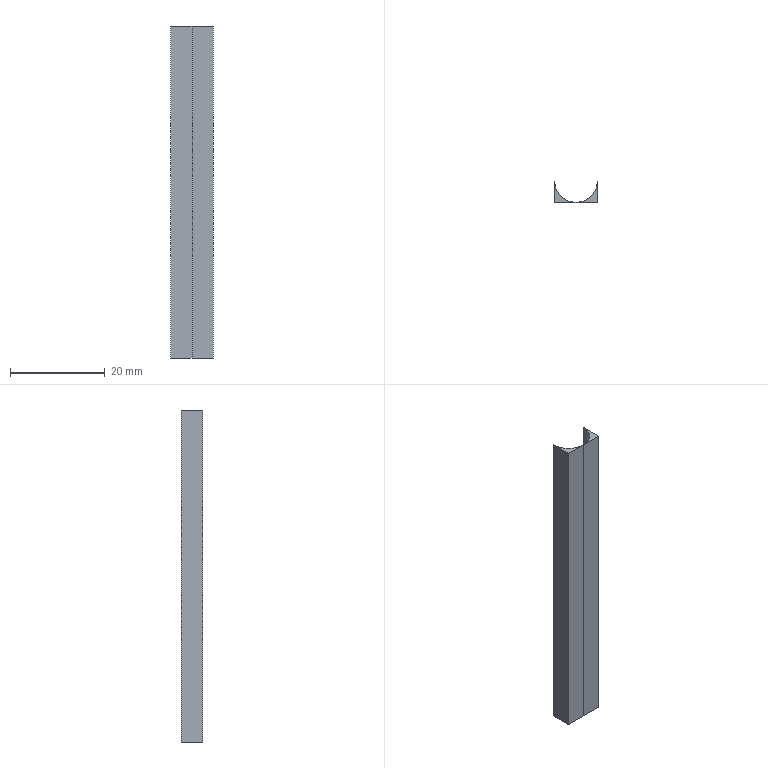Part | STEP file | DCV-000-W03_1 | 2 solids | 10 faces | box 9 x 4.5 x 70 mm | volume 608.396 mm3 | plane 8 | cylinder 2 | commonest cylinder face diameters 9 x2
STEP:
#1=CARTESIAN_POINT('',(0.,0.,0.));
#2=DIRECTION('',(0.,0.,1.));
#3=DIRECTION('',(1.,0.,0.));
#4=AXIS2_PLACEMENT_3D('',#1,#2,#3);
#5=CARTESIAN_POINT('',(0.,-4.5,236.));
#6=VERTEX_POINT('',#5);
#7=CARTESIAN_POINT('',(4.5,0.,236.));
#8=VERTEX_POINT('',#7);
#9=CARTESIAN_POINT('',(0.,0.,236.));
#10=DIRECTION('',(0.,0.,1.));
#11=DIRECTION('',(1.,0.,0.));
#12=AXIS2_PLACEMENT_3D('',#9,#10,#11);
#13=CIRCLE('',#12,4.5);
#14=CARTESIAN_POINT('',(20.,-4.5,236.));
#15=DIRECTION('',(0.,0.,1.));
#16=DIRECTION('',(1.,0.,0.));
#17=AXIS2_PLACEMENT_3D('',#14,#15,#16);
#18=PLANE('',#17);
#19=CARTESIAN_POINT('',(-20.,4.5));
#20=DIRECTION('',(1.,0.));
#21=AXIS2_PLACEMENT_2D('',#19,#20);
#22=CIRCLE('',#21,4.5);
#23=(GEOMETRIC_REPRESENTATION_CONTEXT(2)PARAMETRIC_REPRESENTATION_CONTEXT()REPRESENTATION_CONTEXT('',''));
#24=DEFINITIONAL_REPRESENTATION('',(#22),#23);
#25=PCURVE('',#18,#24);
#26=CARTESIAN_POINT('',(0.,0.,0.));
#27=DIRECTION('',(0.,0.,1.));
#28=DIRECTION('',(1.,0.,0.));
#29=AXIS2_PLACEMENT_3D('',#26,#27,#28);
#30=CYLINDRICAL_SURFACE('',#29,4.5);
#31=CARTESIAN_POINT('',(0.,236.));
#32=DIRECTION('',(1.,0.));
#33=VECTOR('',#32,1.);
#34=LINE('',#31,#33);
#35=(GEOMETRIC_REPRESENTATION_CONTEXT(2)PARAMETRIC_REPRESENTATION_CONTEXT()REPRESENTATION_CONTEXT('',''));
#36=DEFINITIONAL_REPRESENTATION('',(#34),#35);
#37=PCURVE('',#30,#36);
#38=SURFACE_CURVE('',#13,(#25,#37),.PCURVE_S1.);
#39=EDGE_CURVE('',#6,#8,#38,.T.);
#40=ORIENTED_EDGE('',*,*,#39,.F.);
#41=CARTESIAN_POINT('',(4.5,-4.5,236.));
#42=VERTEX_POINT('',#41);
#43=CARTESIAN_POINT('',(25.,-4.5,236.));
#44=DIRECTION('',(-1.,0.,0.));
#45=VECTOR('',#44,1.);
#46=LINE('',#43,#45);
#47=CARTESIAN_POINT('',(5.,0.));
#48=DIRECTION('',(-1.,0.));
#49=VECTOR('',#48,1.);
#50=LINE('',#47,#49);
#51=(GEOMETRIC_REPRESENTATION_CONTEXT(2)PARAMETRIC_REPRESENTATION_CONTEXT()REPRESENTATION_CONTEXT('',''));
#52=DEFINITIONAL_REPRESENTATION('',(#50),#51);
#53=PCURVE('',#18,#52);
#54=CARTESIAN_POINT('',(0.,-4.5,201.));
#55=DIRECTION('',(0.,-1.,0.));
#56=DIRECTION('',(0.,0.,-1.));
#57=AXIS2_PLACEMENT_3D('',#54,#55,#56);
#58=PLANE('',#57);
#59=CARTESIAN_POINT('',(-35.,25.));
#60=DIRECTION('',(0.,-1.));
#61=VECTOR('',#60,1.);
#62=LINE('',#59,#61);
#63=(GEOMETRIC_REPRESENTATION_CONTEXT(2)PARAMETRIC_REPRESENTATION_CONTEXT()REPRESENTATION_CONTEXT('',''));
#64=DEFINITIONAL_REPRESENTATION('',(#62),#63);
#65=PCURVE('',#58,#64);
#66=SURFACE_CURVE('',#46,(#53,#65),.PCURVE_S1.);
#67=EDGE_CURVE('',#42,#6,#66,.T.);
#68=ORIENTED_EDGE('',*,*,#67,.F.);
#69=CARTESIAN_POINT('',(4.5,-2.25,236.));
#70=DIRECTION('',(0.,-1.,0.));
#71=VECTOR('',#70,1.);
#72=LINE('',#69,#71);
#73=CARTESIAN_POINT('',(-15.5,2.25));
#74=DIRECTION('',(0.,-1.));
#75=VECTOR('',#74,1.);
#76=LINE('',#73,#75);
#77=(GEOMETRIC_REPRESENTATION_CONTEXT(2)PARAMETRIC_REPRESENTATION_CONTEXT()REPRESENTATION_CONTEXT('',''));
#78=DEFINITIONAL_REPRESENTATION('',(#76),#77);
#79=PCURVE('',#18,#78);
#80=CARTESIAN_POINT('',(4.5,0.,0.));
#81=DIRECTION('',(1.,0.,0.));
#82=DIRECTION('',(0.,1.,0.));
#83=AXIS2_PLACEMENT_3D('',#80,#81,#82);
#84=PLANE('',#83);
#85=CARTESIAN_POINT('',(-2.25,236.));
#86=DIRECTION('',(-1.,0.));
#87=VECTOR('',#86,1.);
#88=LINE('',#85,#87);
#89=(GEOMETRIC_REPRESENTATION_CONTEXT(2)PARAMETRIC_REPRESENTATION_CONTEXT()REPRESENTATION_CONTEXT('',''));
#90=DEFINITIONAL_REPRESENTATION('',(#88),#89);
#91=PCURVE('',#84,#90);
#92=SURFACE_CURVE('',#72,(#79,#91),.PCURVE_S1.);
#93=EDGE_CURVE('',#8,#42,#92,.T.);
#94=ORIENTED_EDGE('',*,*,#93,.F.);
#95=EDGE_LOOP('',(#40,#68,#94));
#96=FACE_BOUND('',#95,.T.);
#97=ADVANCED_FACE('',(#96),#18,.T.);
#98=CARTESIAN_POINT('',(4.5,-4.5,166.));
#99=VERTEX_POINT('',#98);
#100=CARTESIAN_POINT('',(4.5,-4.5,100.5));
#101=DIRECTION('',(0.,0.,-1.));
#102=VECTOR('',#101,1.);
#103=LINE('',#100,#102);
#104=CARTESIAN_POINT('',(100.5,4.5));
#105=DIRECTION('',(1.,0.));
#106=VECTOR('',#105,1.);
#107=LINE('',#104,#106);
#108=(GEOMETRIC_REPRESENTATION_CONTEXT(2)PARAMETRIC_REPRESENTATION_CONTEXT()REPRESENTATION_CONTEXT('',''));
#109=DEFINITIONAL_REPRESENTATION('',(#107),#108);
#110=PCURVE('',#58,#109);
#111=CARTESIAN_POINT('',(-4.5,100.5));
#112=DIRECTION('',(0.,-1.));
#113=VECTOR('',#112,1.);
#114=LINE('',#111,#113);
#115=(GEOMETRIC_REPRESENTATION_CONTEXT(2)PARAMETRIC_REPRESENTATION_CONTEXT()REPRESENTATION_CONTEXT('',''));
#116=DEFINITIONAL_REPRESENTATION('',(#114),#115);
#117=PCURVE('',#84,#116);
#118=SURFACE_CURVE('',#103,(#110,#117),.PCURVE_S1.);
#119=EDGE_CURVE('',#42,#99,#118,.T.);
#120=ORIENTED_EDGE('',*,*,#119,.F.);
#121=ORIENTED_EDGE('',*,*,#67,.T.);
#122=CARTESIAN_POINT('',(0.,-4.5,166.));
#123=VERTEX_POINT('',#122);
#124=CARTESIAN_POINT('',(0.,-4.5,0.));
#125=DIRECTION('',(0.,0.,1.));
#126=VECTOR('',#125,1.);
#127=LINE('',#124,#126);
#128=CARTESIAN_POINT('',(201.,0.));
#129=DIRECTION('',(-1.,0.));
#130=VECTOR('',#129,1.);
#131=LINE('',#128,#130);
#132=(GEOMETRIC_REPRESENTATION_CONTEXT(2)PARAMETRIC_REPRESENTATION_CONTEXT()REPRESENTATION_CONTEXT('',''));
#133=DEFINITIONAL_REPRESENTATION('',(#131),#132);
#134=PCURVE('',#58,#133);
#135=CARTESIAN_POINT('',(4.712,0.));
#136=DIRECTION('',(0.,1.));
#137=VECTOR('',#136,1.);
#138=LINE('',#135,#137);
#139=(GEOMETRIC_REPRESENTATION_CONTEXT(2)PARAMETRIC_REPRESENTATION_CONTEXT()REPRESENTATION_CONTEXT('',''));
#140=DEFINITIONAL_REPRESENTATION('',(#138),#139);
#141=PCURVE('',#30,#140);
#142=SURFACE_CURVE('',#127,(#134,#141),.PCURVE_S1.);
#143=EDGE_CURVE('',#123,#6,#142,.T.);
#144=ORIENTED_EDGE('',*,*,#143,.F.);
#145=CARTESIAN_POINT('',(-25.,-4.5,166.));
#146=DIRECTION('',(1.,0.,0.));
#147=VECTOR('',#146,1.);
#148=LINE('',#145,#147);
#149=CARTESIAN_POINT('',(35.,-25.));
#150=DIRECTION('',(0.,1.));
#151=VECTOR('',#150,1.);
#152=LINE('',#149,#151);
#153=(GEOMETRIC_REPRESENTATION_CONTEXT(2)PARAMETRIC_REPRESENTATION_CONTEXT()REPRESENTATION_CONTEXT('',''));
#154=DEFINITIONAL_REPRESENTATION('',(#152),#153);
#155=PCURVE('',#58,#154);
#156=CARTESIAN_POINT('',(0.,-4.5,166.));
#157=DIRECTION('',(0.,0.,-1.));
#158=DIRECTION('',(0.,-1.,0.));
#159=AXIS2_PLACEMENT_3D('',#156,#157,#158);
#160=PLANE('',#159);
#161=CARTESIAN_POINT('',(0.,25.));
#162=DIRECTION('',(0.,-1.));
#163=VECTOR('',#162,1.);
#164=LINE('',#161,#163);
#165=(GEOMETRIC_REPRESENTATION_CONTEXT(2)PARAMETRIC_REPRESENTATION_CONTEXT()REPRESENTATION_CONTEXT('',''));
#166=DEFINITIONAL_REPRESENTATION('',(#164),#165);
#167=PCURVE('',#160,#166);
#168=SURFACE_CURVE('',#148,(#155,#167),.PCURVE_S1.);
#169=EDGE_CURVE('',#123,#99,#168,.T.);
#170=ORIENTED_EDGE('',*,*,#169,.T.);
#171=EDGE_LOOP('',(#120,#121,#144,#170));
#172=FACE_BOUND('',#171,.T.);
#173=ADVANCED_FACE('',(#172),#58,.T.);
#174=CARTESIAN_POINT('',(4.5,0.,166.));
#175=VERTEX_POINT('',#174);
#176=CARTESIAN_POINT('',(0.,0.,166.));
#177=DIRECTION('',(0.,0.,-1.));
#178=DIRECTION('',(1.,0.,0.));
#179=AXIS2_PLACEMENT_3D('',#176,#177,#178);
#180=CIRCLE('',#179,4.5);
#181=CARTESIAN_POINT('',(-4.5,0.));
#182=DIRECTION('',(0.,-1.));
#183=AXIS2_PLACEMENT_2D('',#181,#182);
#184=CIRCLE('',#183,4.5);
#185=(GEOMETRIC_REPRESENTATION_CONTEXT(2)PARAMETRIC_REPRESENTATION_CONTEXT()REPRESENTATION_CONTEXT('',''));
#186=DEFINITIONAL_REPRESENTATION('',(#184),#185);
#187=PCURVE('',#160,#186);
#188=CARTESIAN_POINT('',(6.283,166.));
#189=DIRECTION('',(-1.,0.));
#190=VECTOR('',#189,1.);
#191=LINE('',#188,#190);
#192=(GEOMETRIC_REPRESENTATION_CONTEXT(2)PARAMETRIC_REPRESENTATION_CONTEXT()REPRESENTATION_CONTEXT('',''));
#193=DEFINITIONAL_REPRESENTATION('',(#191),#192);
#194=PCURVE('',#30,#193);
#195=SURFACE_CURVE('',#180,(#187,#194),.PCURVE_S1.);
#196=EDGE_CURVE('',#175,#123,#195,.T.);
#197=ORIENTED_EDGE('',*,*,#196,.F.);
#198=CARTESIAN_POINT('',(4.5,-2.25,166.));
#199=DIRECTION('',(0.,1.,0.));
#200=VECTOR('',#199,1.);
#201=LINE('',#198,#200);
#202=CARTESIAN_POINT('',(-2.25,-4.5));
#203=DIRECTION('',(-1.,0.));
#204=VECTOR('',#203,1.);
#205=LINE('',#202,#204);
#206=(GEOMETRIC_REPRESENTATION_CONTEXT(2)PARAMETRIC_REPRESENTATION_CONTEXT()REPRESENTATION_CONTEXT('',''));
#207=DEFINITIONAL_REPRESENTATION('',(#205),#206);
#208=PCURVE('',#160,#207);
#209=CARTESIAN_POINT('',(-2.25,166.));
#210=DIRECTION('',(1.,0.));
#211=VECTOR('',#210,1.);
#212=LINE('',#209,#211);
#213=(GEOMETRIC_REPRESENTATION_CONTEXT(2)PARAMETRIC_REPRESENTATION_CONTEXT()REPRESENTATION_CONTEXT('',''));
#214=DEFINITIONAL_REPRESENTATION('',(#212),#213);
#215=PCURVE('',#84,#214);
#216=SURFACE_CURVE('',#201,(#208,#215),.PCURVE_S1.);
#217=EDGE_CURVE('',#99,#175,#216,.T.);
#218=ORIENTED_EDGE('',*,*,#217,.F.);
#219=ORIENTED_EDGE('',*,*,#169,.F.);
#220=EDGE_LOOP('',(#197,#218,#219));
#221=FACE_BOUND('',#220,.T.);
#222=ADVANCED_FACE('',(#221),#160,.T.);
#223=ORIENTED_EDGE('',*,*,#217,.T.);
#224=CARTESIAN_POINT('',(4.5,0.,0.));
#225=DIRECTION('',(0.,0.,1.));
#226=VECTOR('',#225,1.);
#227=LINE('',#224,#226);
#228=CARTESIAN_POINT('',(0.,0.));
#229=DIRECTION('',(0.,1.));
#230=VECTOR('',#229,1.);
#231=LINE('',#228,#230);
#232=(GEOMETRIC_REPRESENTATION_CONTEXT(2)PARAMETRIC_REPRESENTATION_CONTEXT()REPRESENTATION_CONTEXT('',''));
#233=DEFINITIONAL_REPRESENTATION('',(#231),#232);
#234=PCURVE('',#84,#233);
#235=CARTESIAN_POINT('',(6.283,0.));
#236=DIRECTION('',(0.,1.));
#237=VECTOR('',#236,1.);
#238=LINE('',#235,#237);
#239=(GEOMETRIC_REPRESENTATION_CONTEXT(2)PARAMETRIC_REPRESENTATION_CONTEXT()REPRESENTATION_CONTEXT('',''));
#240=DEFINITIONAL_REPRESENTATION('',(#238),#239);
#241=PCURVE('',#30,#240);
#242=SURFACE_CURVE('',#227,(#234,#241),.PCURVE_S1.);
#243=EDGE_CURVE('',#175,#8,#242,.T.);
#244=ORIENTED_EDGE('',*,*,#243,.T.);
#245=ORIENTED_EDGE('',*,*,#93,.T.);
#246=ORIENTED_EDGE('',*,*,#119,.T.);
#247=EDGE_LOOP('',(#223,#244,#245,#246));
#248=FACE_BOUND('',#247,.T.);
#249=ADVANCED_FACE('',(#248),#84,.T.);
#250=ORIENTED_EDGE('',*,*,#243,.T.);
#251=ORIENTED_EDGE('',*,*,#39,.F.);
#252=ORIENTED_EDGE('',*,*,#143,.F.);
#253=ORIENTED_EDGE('',*,*,#196,.F.);
#254=EDGE_LOOP('',(#250,#251,#252,#253));
#255=FACE_BOUND('',#254,.F.);
#256=ADVANCED_FACE('',(#255),#30,.F.);
#257=CLOSED_SHELL('',(#97,#173,#222,#249,#256));
#258=MANIFOLD_SOLID_BREP('',#257);
#259=CARTESIAN_POINT('',(-4.5,0.,236.));
#260=VERTEX_POINT('',#259);
#261=CARTESIAN_POINT('',(0.,-4.5,236.));
#262=VERTEX_POINT('',#261);
#263=CARTESIAN_POINT('',(0.,0.,236.));
#264=DIRECTION('',(0.,0.,1.));
#265=DIRECTION('',(1.,0.,0.));
#266=AXIS2_PLACEMENT_3D('',#263,#264,#265);
#267=CIRCLE('',#266,4.5);
#268=CARTESIAN_POINT('',(0.,0.,0.));
#269=DIRECTION('',(0.,0.,1.));
#270=DIRECTION('',(1.,0.,0.));
#271=AXIS2_PLACEMENT_3D('',#268,#269,#270);
#272=CYLINDRICAL_SURFACE('',#271,4.5);
#273=CARTESIAN_POINT('',(0.,236.));
#274=DIRECTION('',(1.,0.));
#275=VECTOR('',#274,1.);
#276=LINE('',#273,#275);
#277=(GEOMETRIC_REPRESENTATION_CONTEXT(2)PARAMETRIC_REPRESENTATION_CONTEXT()REPRESENTATION_CONTEXT('',''));
#278=DEFINITIONAL_REPRESENTATION('',(#276),#277);
#279=PCURVE('',#272,#278);
#280=CARTESIAN_POINT('',(0.,-4.5,236.));
#281=DIRECTION('',(0.,0.,1.));
#282=DIRECTION('',(1.,0.,0.));
#283=AXIS2_PLACEMENT_3D('',#280,#281,#282);
#284=PLANE('',#283);
#285=CARTESIAN_POINT('',(0.,4.5));
#286=DIRECTION('',(1.,0.));
#287=AXIS2_PLACEMENT_2D('',#285,#286);
#288=CIRCLE('',#287,4.5);
#289=(GEOMETRIC_REPRESENTATION_CONTEXT(2)PARAMETRIC_REPRESENTATION_CONTEXT()REPRESENTATION_CONTEXT('',''));
#290=DEFINITIONAL_REPRESENTATION('',(#288),#289);
#291=PCURVE('',#284,#290);
#292=SURFACE_CURVE('',#267,(#279,#291),.PCURVE_S1.);
#293=EDGE_CURVE('',#260,#262,#292,.T.);
#294=ORIENTED_EDGE('',*,*,#293,.F.);
#295=CARTESIAN_POINT('',(-4.5,0.,166.));
#296=VERTEX_POINT('',#295);
#297=CARTESIAN_POINT('',(-4.5,0.,0.));
#298=DIRECTION('',(0.,0.,-1.));
#299=VECTOR('',#298,1.);
#300=LINE('',#297,#299);
#301=CARTESIAN_POINT('',(3.142,0.));
#302=DIRECTION('',(0.,-1.));
#303=VECTOR('',#302,1.);
#304=LINE('',#301,#303);
#305=(GEOMETRIC_REPRESENTATION_CONTEXT(2)PARAMETRIC_REPRESENTATION_CONTEXT()REPRESENTATION_CONTEXT('',''));
#306=DEFINITIONAL_REPRESENTATION('',(#304),#305);
#307=PCURVE('',#272,#306);
#308=CARTESIAN_POINT('',(-4.5,0.,236.));
#309=DIRECTION('',(-1.,0.,0.));
#310=DIRECTION('',(0.,0.,1.));
#311=AXIS2_PLACEMENT_3D('',#308,#309,#310);
#312=PLANE('',#311);
#313=CARTESIAN_POINT('',(-236.,0.));
#314=DIRECTION('',(-1.,0.));
#315=VECTOR('',#314,1.);
#316=LINE('',#313,#315);
#317=(GEOMETRIC_REPRESENTATION_CONTEXT(2)PARAMETRIC_REPRESENTATION_CONTEXT()REPRESENTATION_CONTEXT('',''));
#318=DEFINITIONAL_REPRESENTATION('',(#316),#317);
#319=PCURVE('',#312,#318);
#320=SURFACE_CURVE('',#300,(#307,#319),.PCURVE_S1.);
#321=EDGE_CURVE('',#260,#296,#320,.T.);
#322=ORIENTED_EDGE('',*,*,#321,.T.);
#323=CARTESIAN_POINT('',(0.,-4.5,166.));
#324=VERTEX_POINT('',#323);
#325=CARTESIAN_POINT('',(0.,0.,166.));
#326=DIRECTION('',(0.,0.,-1.));
#327=DIRECTION('',(1.,0.,0.));
#328=AXIS2_PLACEMENT_3D('',#325,#326,#327);
#329=CIRCLE('',#328,4.5);
#330=CARTESIAN_POINT('',(6.283,166.));
#331=DIRECTION('',(-1.,0.));
#332=VECTOR('',#331,1.);
#333=LINE('',#330,#332);
#334=(GEOMETRIC_REPRESENTATION_CONTEXT(2)PARAMETRIC_REPRESENTATION_CONTEXT()REPRESENTATION_CONTEXT('',''));
#335=DEFINITIONAL_REPRESENTATION('',(#333),#334);
#336=PCURVE('',#272,#335);
#337=CARTESIAN_POINT('',(-20.,-4.5,166.));
#338=DIRECTION('',(0.,0.,-1.));
#339=DIRECTION('',(0.,-1.,0.));
#340=AXIS2_PLACEMENT_3D('',#337,#338,#339);
#341=PLANE('',#340);
#342=CARTESIAN_POINT('',(-4.5,-20.));
#343=DIRECTION('',(0.,-1.));
#344=AXIS2_PLACEMENT_2D('',#342,#343);
#345=CIRCLE('',#344,4.5);
#346=(GEOMETRIC_REPRESENTATION_CONTEXT(2)PARAMETRIC_REPRESENTATION_CONTEXT()REPRESENTATION_CONTEXT('',''));
#347=DEFINITIONAL_REPRESENTATION('',(#345),#346);
#348=PCURVE('',#341,#347);
#349=SURFACE_CURVE('',#329,(#336,#348),.PCURVE_S1.);
#350=EDGE_CURVE('',#324,#296,#349,.T.);
#351=ORIENTED_EDGE('',*,*,#350,.F.);
#352=CARTESIAN_POINT('',(0.,-4.5,0.));
#353=DIRECTION('',(0.,0.,1.));
#354=VECTOR('',#353,1.);
#355=LINE('',#352,#354);
#356=CARTESIAN_POINT('',(4.712,0.));
#357=DIRECTION('',(0.,1.));
#358=VECTOR('',#357,1.);
#359=LINE('',#356,#358);
#360=(GEOMETRIC_REPRESENTATION_CONTEXT(2)PARAMETRIC_REPRESENTATION_CONTEXT()REPRESENTATION_CONTEXT('',''));
#361=DEFINITIONAL_REPRESENTATION('',(#359),#360);
#362=PCURVE('',#272,#361);
#363=CARTESIAN_POINT('',(0.,-4.5,201.));
#364=DIRECTION('',(0.,-1.,0.));
#365=DIRECTION('',(0.,0.,-1.));
#366=AXIS2_PLACEMENT_3D('',#363,#364,#365);
#367=PLANE('',#366);
#368=CARTESIAN_POINT('',(201.,0.));
#369=DIRECTION('',(-1.,0.));
#370=VECTOR('',#369,1.);
#371=LINE('',#368,#370);
#372=(GEOMETRIC_REPRESENTATION_CONTEXT(2)PARAMETRIC_REPRESENTATION_CONTEXT()REPRESENTATION_CONTEXT('',''));
#373=DEFINITIONAL_REPRESENTATION('',(#371),#372);
#374=PCURVE('',#367,#373);
#375=SURFACE_CURVE('',#355,(#362,#374),.PCURVE_S1.);
#376=EDGE_CURVE('',#324,#262,#375,.T.);
#377=ORIENTED_EDGE('',*,*,#376,.T.);
#378=EDGE_LOOP('',(#294,#322,#351,#377));
#379=FACE_BOUND('',#378,.F.);
#380=ADVANCED_FACE('',(#379),#272,.F.);
#381=CARTESIAN_POINT('',(-4.5,-4.5,166.));
#382=VERTEX_POINT('',#381);
#383=CARTESIAN_POINT('',(-4.5,-4.5,236.));
#384=VERTEX_POINT('',#383);
#385=CARTESIAN_POINT('',(-4.5,-4.5,218.5));
#386=DIRECTION('',(0.,0.,1.));
#387=VECTOR('',#386,1.);
#388=LINE('',#385,#387);
#389=CARTESIAN_POINT('',(-17.5,-4.5));
#390=DIRECTION('',(1.,0.));
#391=VECTOR('',#390,1.);
#392=LINE('',#389,#391);
#393=(GEOMETRIC_REPRESENTATION_CONTEXT(2)PARAMETRIC_REPRESENTATION_CONTEXT()REPRESENTATION_CONTEXT('',''));
#394=DEFINITIONAL_REPRESENTATION('',(#392),#393);
#395=PCURVE('',#312,#394);
#396=CARTESIAN_POINT('',(-17.5,-4.5));
#397=DIRECTION('',(-1.,0.));
#398=VECTOR('',#397,1.);
#399=LINE('',#396,#398);
#400=(GEOMETRIC_REPRESENTATION_CONTEXT(2)PARAMETRIC_REPRESENTATION_CONTEXT()REPRESENTATION_CONTEXT('',''));
#401=DEFINITIONAL_REPRESENTATION('',(#399),#400);
#402=PCURVE('',#367,#401);
#403=SURFACE_CURVE('',#388,(#395,#402),.PCURVE_S1.);
#404=EDGE_CURVE('',#382,#384,#403,.T.);
#405=ORIENTED_EDGE('',*,*,#404,.T.);
#406=CARTESIAN_POINT('',(-4.5,-2.25,236.));
#407=DIRECTION('',(0.,1.,0.));
#408=VECTOR('',#407,1.);
#409=LINE('',#406,#408);
#410=CARTESIAN_POINT('',(0.,-2.25));
#411=DIRECTION('',(0.,1.));
#412=VECTOR('',#411,1.);
#413=LINE('',#410,#412);
#414=(GEOMETRIC_REPRESENTATION_CONTEXT(2)PARAMETRIC_REPRESENTATION_CONTEXT()REPRESENTATION_CONTEXT('',''));
#415=DEFINITIONAL_REPRESENTATION('',(#413),#414);
#416=PCURVE('',#312,#415);
#417=CARTESIAN_POINT('',(-4.5,2.25));
#418=DIRECTION('',(0.,1.));
#419=VECTOR('',#418,1.);
#420=LINE('',#417,#419);
#421=(GEOMETRIC_REPRESENTATION_CONTEXT(2)PARAMETRIC_REPRESENTATION_CONTEXT()REPRESENTATION_CONTEXT('',''));
#422=DEFINITIONAL_REPRESENTATION('',(#420),#421);
#423=PCURVE('',#284,#422);
#424=SURFACE_CURVE('',#409,(#416,#423),.PCURVE_S1.);
#425=EDGE_CURVE('',#384,#260,#424,.T.);
#426=ORIENTED_EDGE('',*,*,#425,.T.);
#427=ORIENTED_EDGE('',*,*,#321,.T.);
#428=CARTESIAN_POINT('',(-4.5,-2.25,166.));
#429=DIRECTION('',(0.,-1.,0.));
#430=VECTOR('',#429,1.);
#431=LINE('',#428,#430);
#432=CARTESIAN_POINT('',(-70.,-2.25));
#433=DIRECTION('',(0.,-1.));
#434=VECTOR('',#433,1.);
#435=LINE('',#432,#434);
#436=(GEOMETRIC_REPRESENTATION_CONTEXT(2)PARAMETRIC_REPRESENTATION_CONTEXT()REPRESENTATION_CONTEXT('',''));
#437=DEFINITIONAL_REPRESENTATION('',(#435),#436);
#438=PCURVE('',#312,#437);
#439=CARTESIAN_POINT('',(-2.25,-15.5));
#440=DIRECTION('',(1.,0.));
#441=VECTOR('',#440,1.);
#442=LINE('',#439,#441);
#443=(GEOMETRIC_REPRESENTATION_CONTEXT(2)PARAMETRIC_REPRESENTATION_CONTEXT()REPRESENTATION_CONTEXT('',''));
#444=DEFINITIONAL_REPRESENTATION('',(#442),#443);
#445=PCURVE('',#341,#444);
#446=SURFACE_CURVE('',#431,(#438,#445),.PCURVE_S1.);
#447=EDGE_CURVE('',#296,#382,#446,.T.);
#448=ORIENTED_EDGE('',*,*,#447,.T.);
#449=EDGE_LOOP('',(#405,#426,#427,#448));
#450=FACE_BOUND('',#449,.T.);
#451=ADVANCED_FACE('',(#450),#312,.T.);
#452=ORIENTED_EDGE('',*,*,#293,.F.);
#453=ORIENTED_EDGE('',*,*,#425,.F.);
#454=CARTESIAN_POINT('',(25.,-4.5,236.));
#455=DIRECTION('',(-1.,0.,0.));
#456=VECTOR('',#455,1.);
#457=LINE('',#454,#456);
#458=CARTESIAN_POINT('',(25.,0.));
#459=DIRECTION('',(-1.,0.));
#460=VECTOR('',#459,1.);
#461=LINE('',#458,#460);
#462=(GEOMETRIC_REPRESENTATION_CONTEXT(2)PARAMETRIC_REPRESENTATION_CONTEXT()REPRESENTATION_CONTEXT('',''));
#463=DEFINITIONAL_REPRESENTATION('',(#461),#462);
#464=PCURVE('',#284,#463);
#465=CARTESIAN_POINT('',(-35.,25.));
#466=DIRECTION('',(0.,-1.));
#467=VECTOR('',#466,1.);
#468=LINE('',#465,#467);
#469=(GEOMETRIC_REPRESENTATION_CONTEXT(2)PARAMETRIC_REPRESENTATION_CONTEXT()REPRESENTATION_CONTEXT('',''));
#470=DEFINITIONAL_REPRESENTATION('',(#468),#469);
#471=PCURVE('',#367,#470);
#472=SURFACE_CURVE('',#457,(#464,#471),.PCURVE_S1.);
#473=EDGE_CURVE('',#262,#384,#472,.T.);
#474=ORIENTED_EDGE('',*,*,#473,.F.);
#475=EDGE_LOOP('',(#452,#453,#474));
#476=FACE_BOUND('',#475,.T.);
#477=ADVANCED_FACE('',(#476),#284,.T.);
#478=ORIENTED_EDGE('',*,*,#404,.F.);
#479=CARTESIAN_POINT('',(-25.,-4.5,166.));
#480=DIRECTION('',(1.,0.,0.));
#481=VECTOR('',#480,1.);
#482=LINE('',#479,#481);
#483=CARTESIAN_POINT('',(35.,-25.));
#484=DIRECTION('',(0.,1.));
#485=VECTOR('',#484,1.);
#486=LINE('',#483,#485);
#487=(GEOMETRIC_REPRESENTATION_CONTEXT(2)PARAMETRIC_REPRESENTATION_CONTEXT()REPRESENTATION_CONTEXT('',''));
#488=DEFINITIONAL_REPRESENTATION('',(#486),#487);
#489=PCURVE('',#367,#488);
#490=CARTESIAN_POINT('',(0.,5.));
#491=DIRECTION('',(0.,-1.));
#492=VECTOR('',#491,1.);
#493=LINE('',#490,#492);
#494=(GEOMETRIC_REPRESENTATION_CONTEXT(2)PARAMETRIC_REPRESENTATION_CONTEXT()REPRESENTATION_CONTEXT('',''));
#495=DEFINITIONAL_REPRESENTATION('',(#493),#494);
#496=PCURVE('',#341,#495);
#497=SURFACE_CURVE('',#482,(#489,#496),.PCURVE_S1.);
#498=EDGE_CURVE('',#382,#324,#497,.T.);
#499=ORIENTED_EDGE('',*,*,#498,.T.);
#500=ORIENTED_EDGE('',*,*,#376,.T.);
#501=ORIENTED_EDGE('',*,*,#473,.T.);
#502=EDGE_LOOP('',(#478,#499,#500,#501));
#503=FACE_BOUND('',#502,.T.);
#504=ADVANCED_FACE('',(#503),#367,.T.);
#505=ORIENTED_EDGE('',*,*,#350,.F.);
#506=ORIENTED_EDGE('',*,*,#498,.F.);
#507=ORIENTED_EDGE('',*,*,#447,.F.);
#508=EDGE_LOOP('',(#505,#506,#507));
#509=FACE_BOUND('',#508,.T.);
#510=ADVANCED_FACE('',(#509),#341,.T.);
#511=CLOSED_SHELL('',(#380,#451,#477,#504,#510));
#512=MANIFOLD_SOLID_BREP('',#511);
#513=(LENGTH_UNIT()NAMED_UNIT(*)SI_UNIT(.MILLI.,.METRE.));
#514=UNCERTAINTY_MEASURE_WITH_UNIT(LENGTH_MEASURE(0.0000001),#513,'','');
#515=(NAMED_UNIT(*)PLANE_ANGLE_UNIT()SI_UNIT($,.RADIAN.));
#516=(NAMED_UNIT(*)SI_UNIT($,.STERADIAN.)SOLID_ANGLE_UNIT());
#517=(GEOMETRIC_REPRESENTATION_CONTEXT(3)GLOBAL_UNCERTAINTY_ASSIGNED_CONTEXT((#514))GLOBAL_UNIT_ASSIGNED_CONTEXT((#513,#515,#516))REPRESENTATION_CONTEXT('',''));
#518=SHAPE_REPRESENTATION('',(#4,#258,#512),#517);